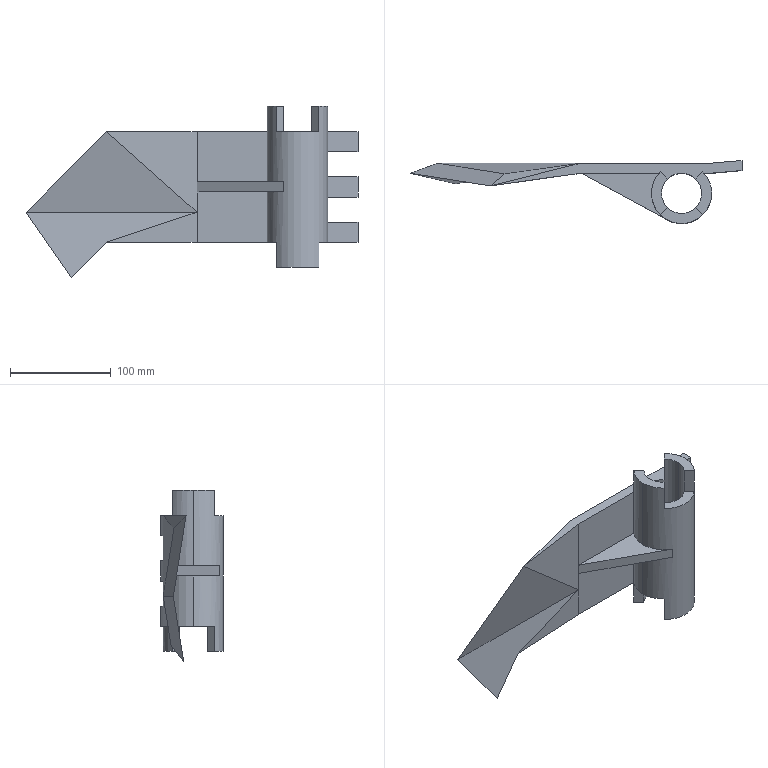Part | SolidWorks | features ICE 14, Extrusion 1, Rib 1 | 1 solid | 57 faces | box 330 x 62.625 x 170 mm | volume 487864 mm3 | plane 50 | cylinder 7 | commonest cylinder face diameters 60 x5 40 x2